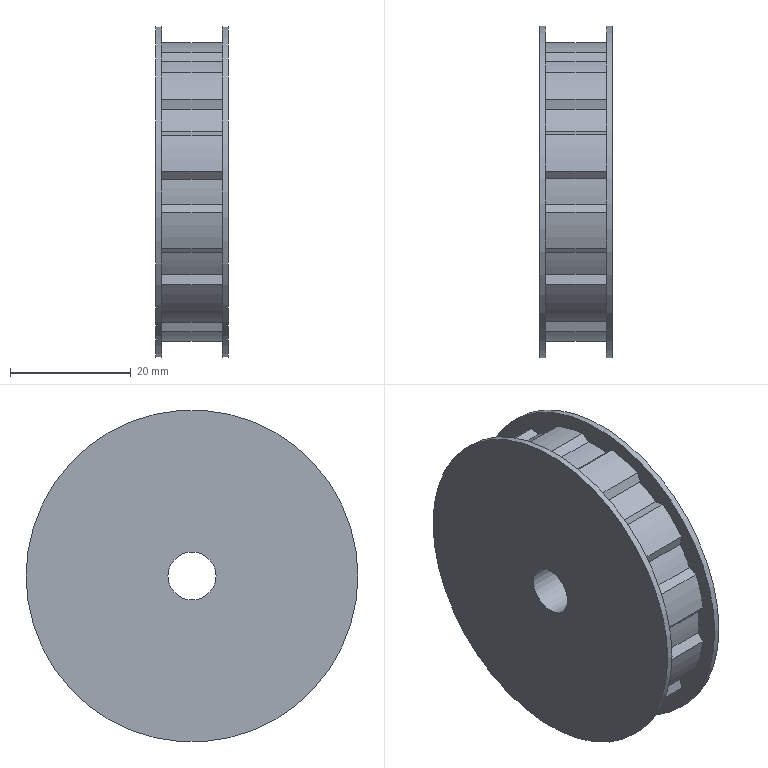Part | NX | features DATUM_CSYS 3, EXTRUDE 2, SKETCH 2, Container 1, EXTRACT_BODY 1, Geometry Instance 1, UNITE 1 | 1 solid | 55 faces | box 12 x 55 x 55 mm | volume 22955 mm3 | plane 28 | cylinder 27 | commonest cylinder face diameters 47.525 x12 50 x12 55 x2 8 x1